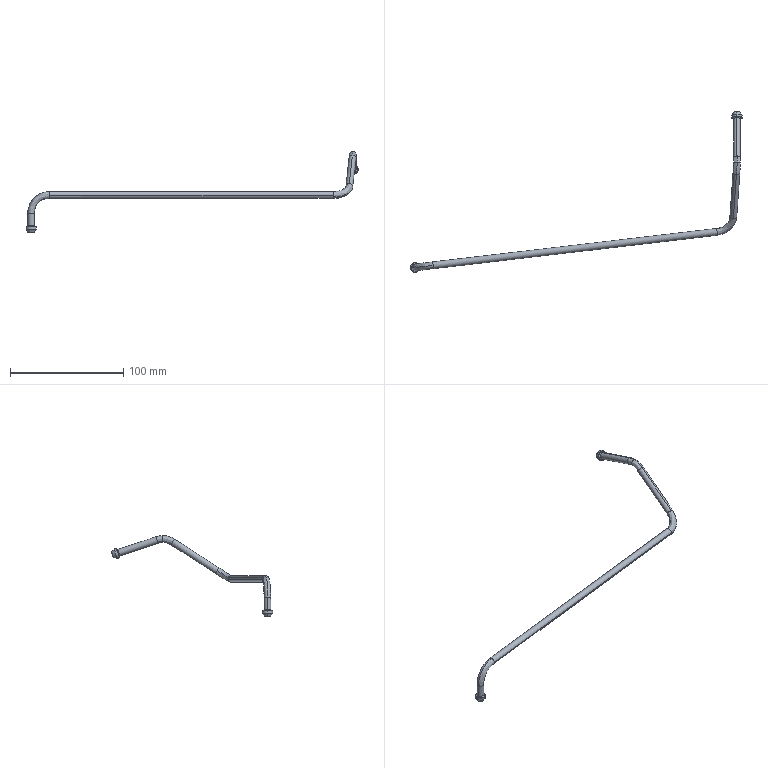Part | SolidWorks | features BaseBody 1 | 1 solid | 60 faces | box 293 x 142.113 x 71.383 mm | volume 11329 mm3 | cylinder 24 | spline 20 | cone 12 | plane 4 | commonest cylinder face diameters 1.5 x8 6 x8 2 x4 9 x4